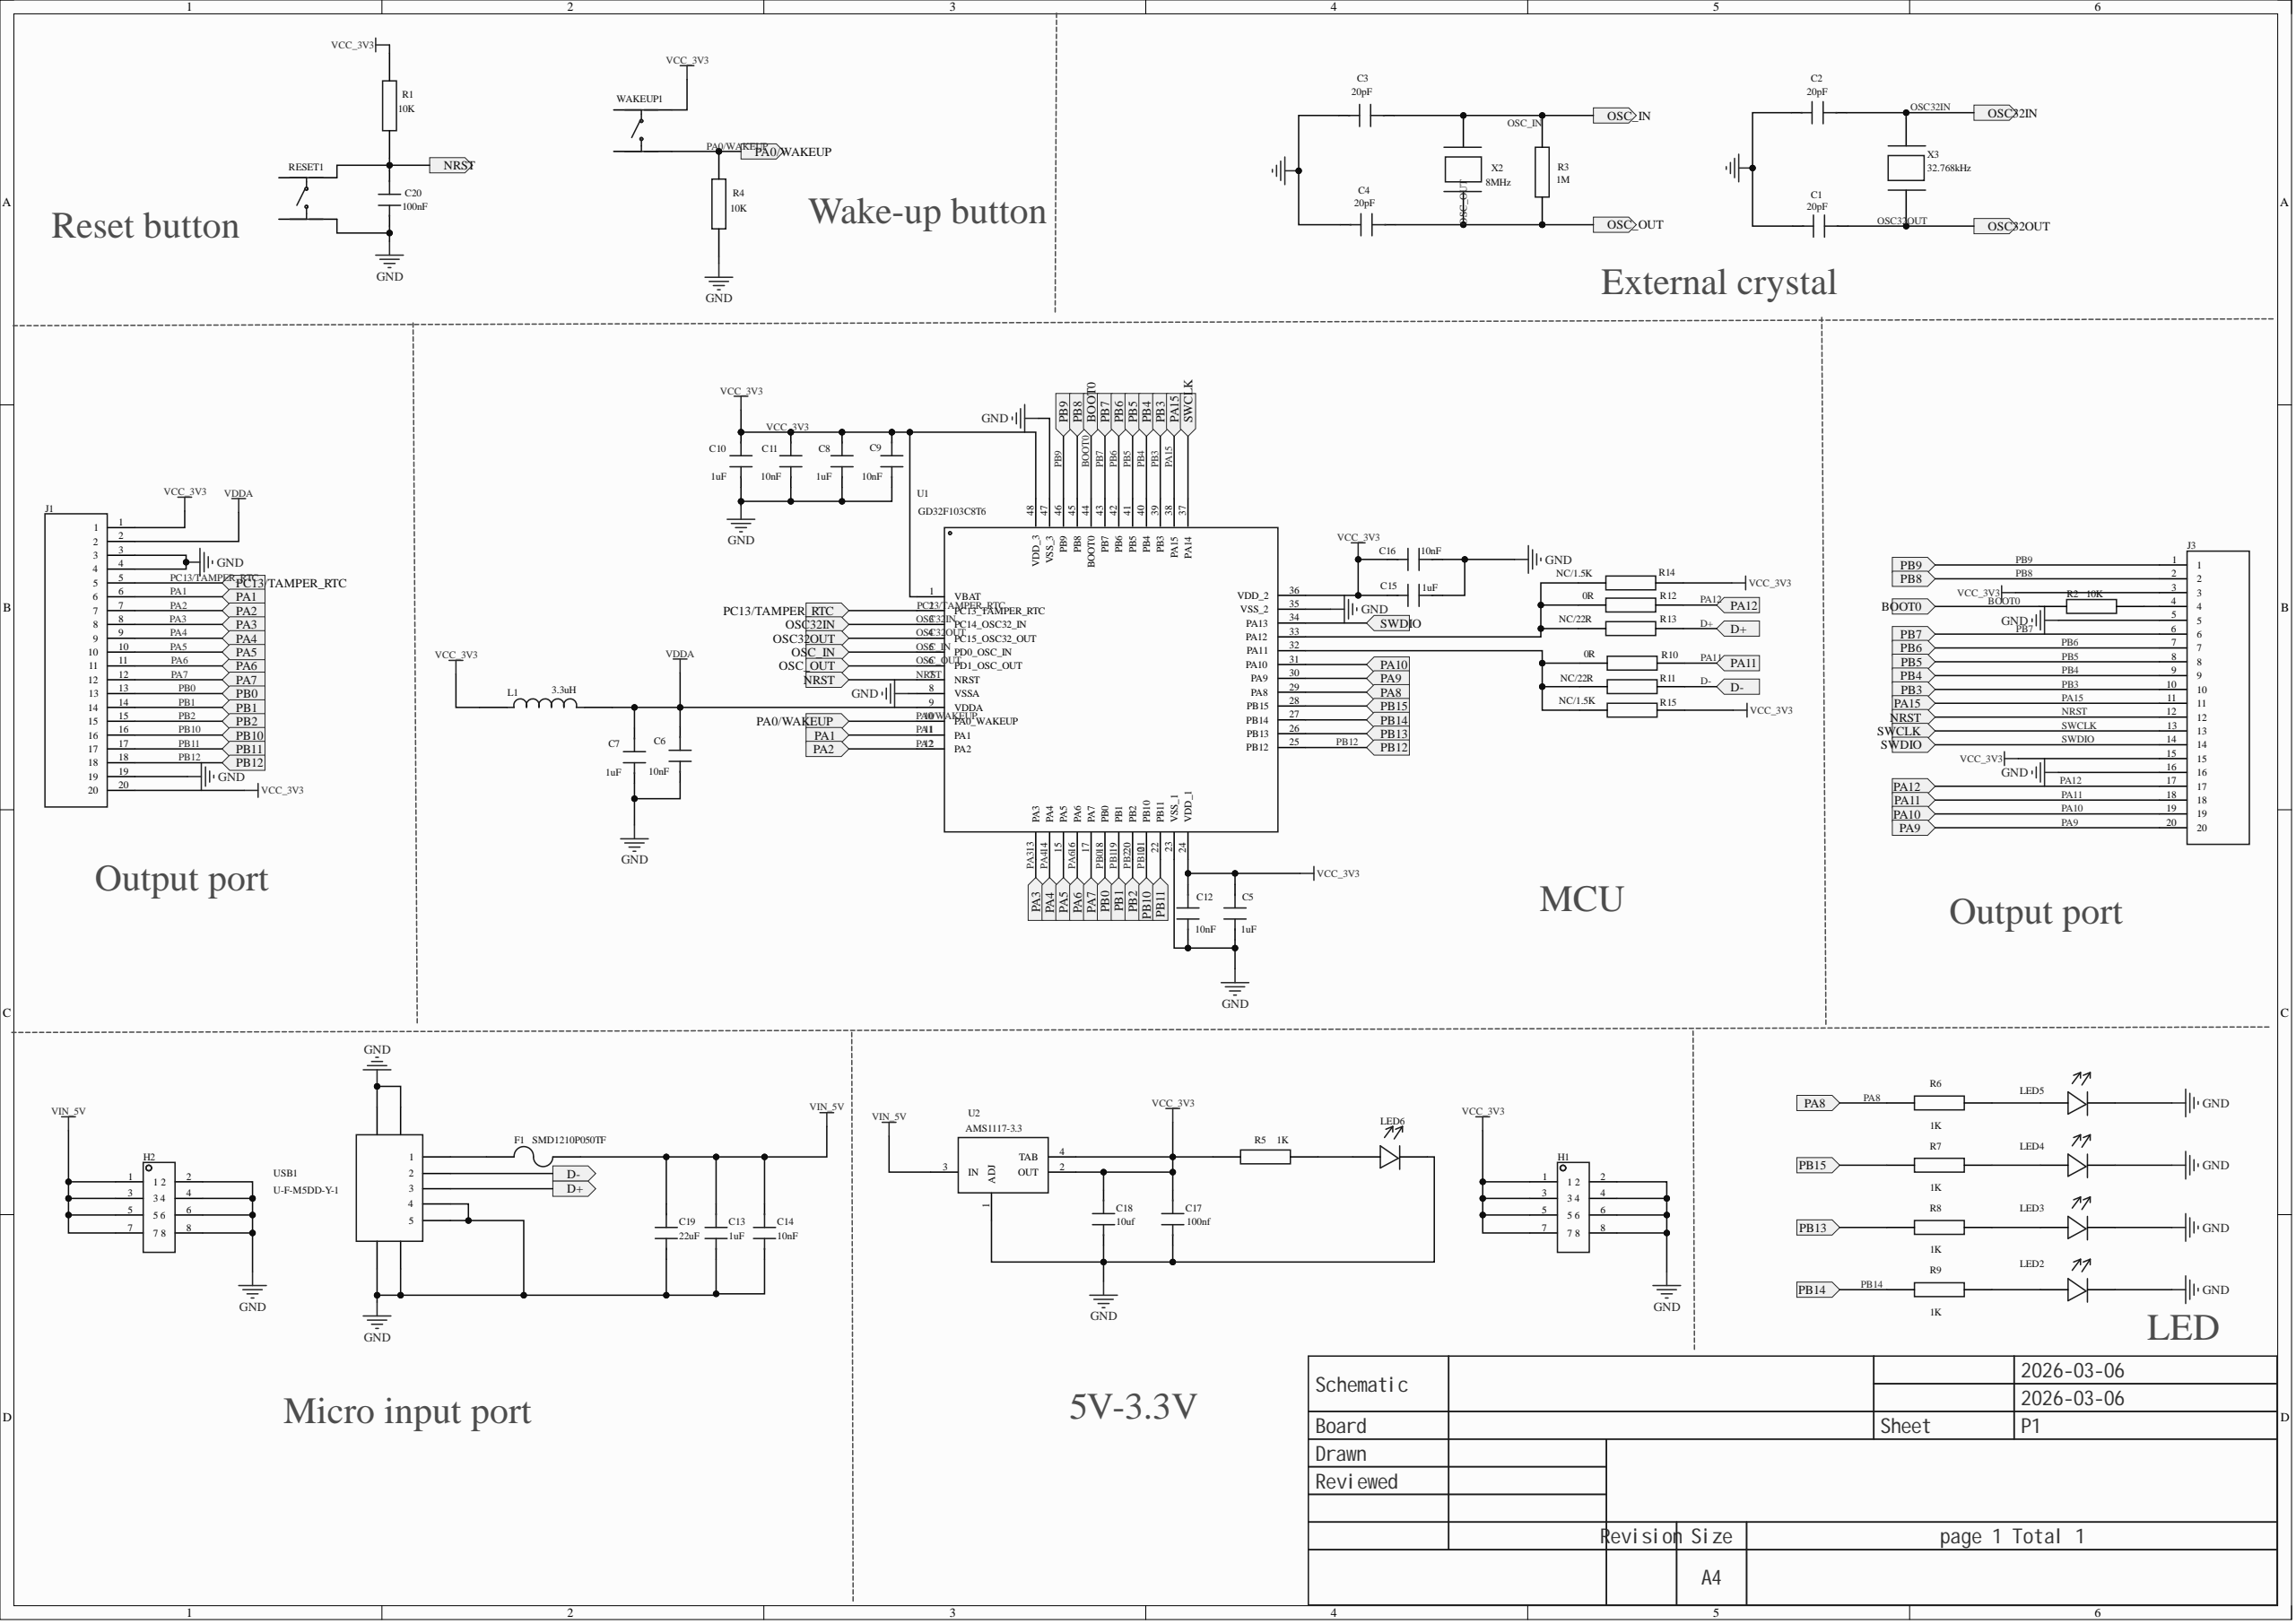Circuit board | Altium Designer | 53 parts | 54 nets
Bill of materials:
Comment,Description,Designator,Footprint,LibRef,Quantity
"20pF","","C1, C2, C3, C4","C0603","C","4"
"1uF","","C5, C7, C8, C10, C13, C15","C0603","C","6"
"10nF","","C6, C9, C11, C12, C14, C16","C0603","C","6"
"100nf","","C17, C20","C0603","C","2"
"10uf","","C18","C0805","C","1"
"22uF","","C19","C0805","C","1"
"","","F1","F1210","SMD1210P050TF","1"
"","","H1, H2","HDR-TH_8P-P2.54-V-M-R2-C4-S2.54","PZ254V-12-8P","2"
"","","J1, J3","HDR-TH_20PIN-V-MALE-PITCH2.54","HDR-20P","2"
"3.3uH","","L1","L0603","L","1"
"","","LED2, LED3, LED4, LED5, LED6","LED0603","LED","5"
"10K","Resistor","R1, R2, R4","R0603","R","3"
"1M","Resistor","R3","R0603","R","1"
"1K","Resistor","R5, R6, R7, R8, R9","R0603","R","5"
"0R","Resistor","R10, R12","R0603","R","2"
"NC/22R","Resistor","R11, R13","R0603","R","2"
"NC/1.5K","Resistor","R14, R15","R0603","R","2"
"","","RESET1, WAKEUP1","SW-SMD-T6X6-9.5X5.8","TSA063G43-250","2"
"","","U1","TQFP-48_L7.0-W7.0-P0.50-LS9.0-BL","GD32F103C8T6","1"
"","","U2","SOT-223","AMS1117-3.3","1"
"","","USB1","U-F-M5DD-Y-1","U-F-M5DD-Y-1","1"
"8MHz","","X2","OSC-49S-1","晶振","1"
"32.768kHz","","X3","DT-38_BD3.1-P0.80","晶振","1"
Netlist (Protel format):
[
C1
C0603
20pF



]
[
C2
C0603
20pF



]
[
C3
C0603
20pF



]
[
C4
C0603
20pF



]
[
C5
C0603
1uF



]
[
C6
C0603
10nF



]
[
C7
C0603
1uF



]
[
C8
C0603
1uF



]
[
C9
C0603
10nF



]
[
C10
C0603
1uF



]
[
C11
C0603
10nF



]
[
C12
C0603
10nF



]
[
C13
C0603
1uF



]
[
C14
C0603
10nF



]
[
C15
C0603
1uF



]
[
C16
C0603
10nF



]
[
C17
C0603
100nf



]
[
C18
C0805
10uf



]
[
C19
C0805
22uF



]
[
C20
C0603
100nF



]
[
F1
F1210




]
[
H1
HDR-TH_8P-P2.54-V-M-R2-C4-S2.54




]
[
H2
HDR-TH_8P-P2.54-V-M-R2-C4-S2.54




]
[
J1
HDR-TH_20PIN-V-MALE-PITCH2.54




]
[
J3
HDR-TH_20PIN-V-MALE-PITCH2.54




]
[
L1
L0603
3.3uH



]
[
LED2
LED0603




]
[
LED3
LED0603




]
[
LED4
LED0603




]
[
LED5
LED0603




]
[
LED6
LED0603




]
[
R1
R0603
10K



]
[
R2
R0603
10K



]
[
R3
R0603
1M



]
[
R4
R0603
10K



]
[
R5
R0603
1K



]
[
R6
R0603
1K



]
[
R7
R0603
1K



]
[
R8
R0603
1K



]
[
R9
R0603
1K



]
[
R10
R0603
0R



]
[
R11
R0603
NC/22R



]
[
R12
R0603
0R



]
[
R13
R0603
NC/22R



]
[
R14
R0603
NC/1.5K



]
[
R15
R0603
NC/1.5K



]
[
RESET1
SW-SMD-T6X6-9.5X5.8




]
[
U1
TQFP-48_L7.0-W7.0-P0.50-LS9.0-BL




]
[
U2
SOT-223




]
[
USB1
U-F-M5DD-Y-1




]
[
WAKEUP1
SW-SMD-T6X6-9.5X5.8




]
[
X2
OSC-49S-1
8MHz



]
[
X3
DT-38_BD3.1-P0.80
32.768kHz



]
(
VIN_5V
C13-2
C14-2
C19-2
F1-2
H2-1
H2-3
H2-5
H2-7
U2-3
)
(
VDDA
C6-2
C7-2
J1-2
L1-2
U1-9
)
(
VCC_3V3
C5-2
C8-2
C9-2
C10-2
C11-2
C12-2
C15-1
C16-1
C17-2
C18-2
H1-1
H1-3
H1-5
H1-7
J1-1
J1-20
J3-3
J3-15
L1-1
R1-2
R5-1
R14-2
R15-2
U1-1
U1-24
U1-36
U1-48
U2-2
U2-4
WAKEUP1-1
)
(
SWDIO
J3-14
U1-34
)
(
SWCLK
J3-13
U1-37
)
(
PC13/TAMPER_RTC
J1-5
U1-2
)
(
PB14
R9-1
U1-27
)
(
PB12
J1-18
U1-25
)
(
PB11
J1-17
U1-22
)
(
PB10
J1-16
U1-21
)
(
PB9
J3-1
U1-46
)
(
PB8
J3-2
U1-45
)
(
PB7
J3-6
U1-43
)
(
PB6
J3-7
U1-42
)
(
PB5
J3-8
U1-41
)
(
PB4
J3-9
U1-40
)
(
PB3
J3-10
U1-39
)
(
PB2
J1-15
U1-20
)
(
PB1
J1-14
U1-19
)
(
PB0
J1-13
U1-18
)
(
PA15
J3-11
U1-38
)
(
PA12
J3-17
R12-2
)
(
PA11
J3-18
R10-2
)
(
PA10
J3-19
U1-31
)
(
PA9
J3-20
U1-30
)
(
PA8
R6-1
U1-29
)
(
PA7
J1-12
U1-17
)
(
PA6
J1-11
U1-16
)
(
PA5
J1-10
U1-15
)
(
PA4
J1-9
U1-14
)
(
PA3
J1-8
U1-13
)
(
PA2
J1-7
U1-12
)
(
PA1
J1-6
U1-11
)
(
PA0/WAKEUP
R4-2
U1-10
WAKEUP1-3
)
(
OSC_OUT
C4-2
R3-1
U1-6
X2-1
)
(
OSC_IN
C3-2
R3-2
U1-5
X2-2
)
(
OSC32OUT
C1-2
U1-4
X3-2
)
(
OSC32IN
C2-2
U1-3
X3-1
)
(
NRST
C20-2
J3-12
R1-1
RESET1-1
U1-7
)
(
NetR12_1
R12-1
R13-1
R14-1
U1-33
)
(
NetR10_1
R10-1
R11-1
R15-1
U1-32
)
(
NetR8_1
R8-1
U1-26
)
(
NetR7_1
R7-1
U1-28
)
(
NetLED6_2
LED6-2
R5-2
)
(
NetLED5_2
LED5-2
R6-2
)
(
NetLED4_2
LED4-2
R7-2
)
(
NetLED3_2
LED3-2
R8-2
)
(
NetLED2_2
LED2-2
R9-2
)
(
NetJ3_4
J3-4
R2-2
)
(
NetF1_1
F1-1
USB1-1
)
(
GND
C1-1
C2-1
C3-1
C4-1
C5-1
C6-1
C7-1
C8-1
C9-1
C10-1
C11-1
C12-1
C13-1
C14-1
C15-2
C16-2
C17-1
C18-1
C19-1
C20-1
H1-2
H1-4
H1-6
H1-8
H2-2
H2-4
H2-6
H2-8
J1-3
J1-4
J1-19
J3-5
J3-16
LED2-1
LED3-1
LED4-1
LED5-1
LED6-1
R4-1
RESET1-3
U1-8
U1-23
U1-35
U1-47
U2-1
USB1-4
USB1-5
USB1-6
USB1-7
USB1-8
USB1-9
)
(
D-
R11-2
USB1-2
)
(
D+
R13-2
USB1-3
)
(
BOOT0
R2-1
U1-44
)